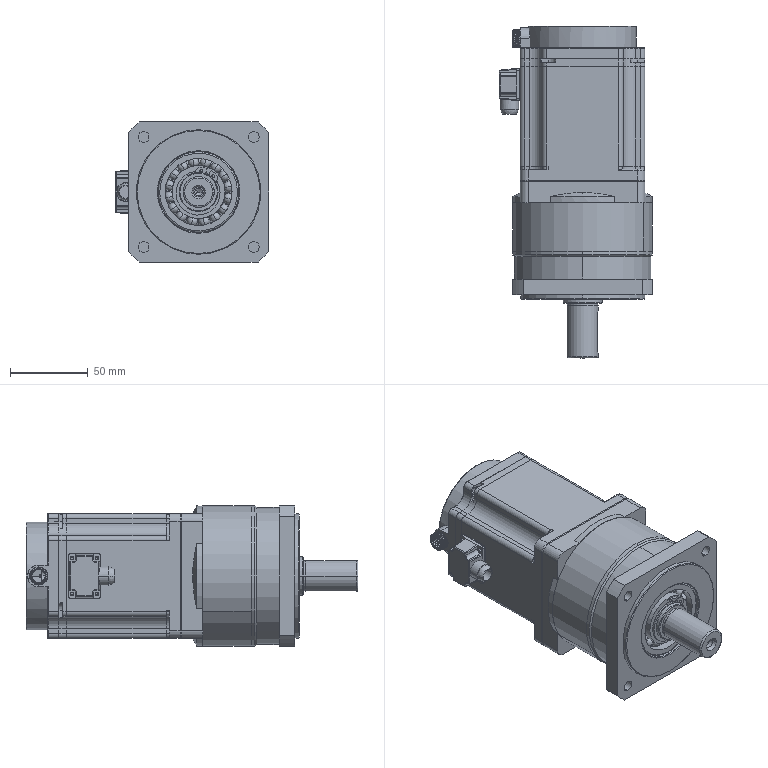Part | STEP file | YBQDJ-PD-2 | 28 solids | 3428 faces | volume 675014 mm3 | cylinder 1503 | plane 776 | spline 488 | torus 289 | cone 242 | sphere 130 | commonest cylinder face diameters 1.5 x156 63.9 x109 66.54 x108 14.94 x81 17.4 x81 0.752 x61